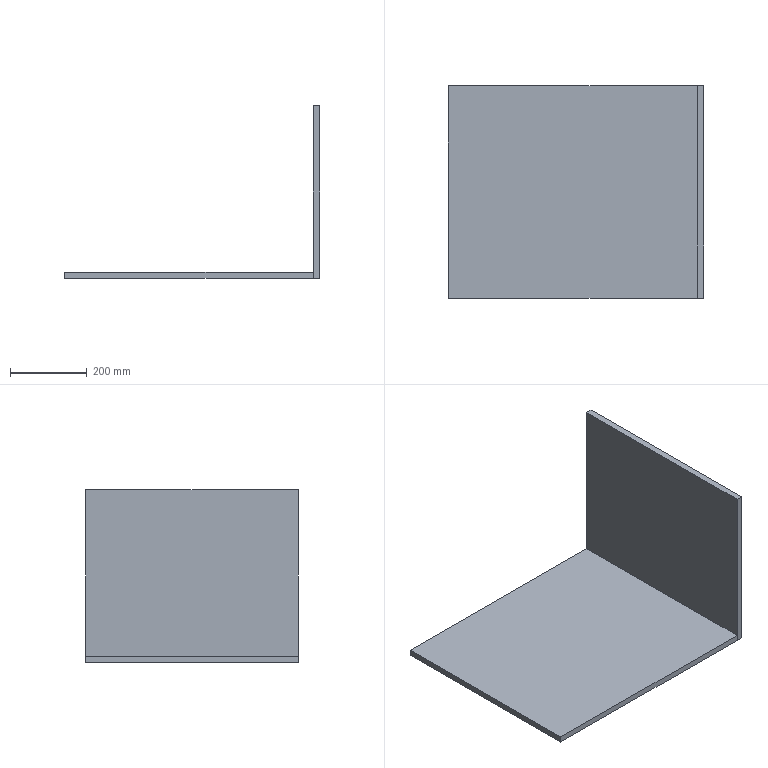Part | SolidWorks | features BaseBody 2 | 2 solids | 12 faces | box 666 x 555 x 451 mm | volume 9776880 mm3 | plane 12
STEP:
#1=CARTESIAN_POINT('',(325.,277.5,0.));
#2=VERTEX_POINT('',#1);
#3=CARTESIAN_POINT('',(-325.,277.5,0.));
#4=VERTEX_POINT('',#3);
#5=CARTESIAN_POINT('',(325.,277.5,0.));
#6=DIRECTION('',(-1.,0.,0.));
#7=VECTOR('',#6,1000.);
#8=LINE('',#5,#7);
#9=EDGE_CURVE('',#2,#4,#8,.T.);
#10=ORIENTED_EDGE('',*,*,#9,.F.);
#11=CARTESIAN_POINT('',(325.,-277.5,0.));
#12=VERTEX_POINT('',#11);
#13=CARTESIAN_POINT('',(325.,-277.5,0.));
#14=DIRECTION('',(0.,1.,0.));
#15=VECTOR('',#14,1000.);
#16=LINE('',#13,#15);
#17=EDGE_CURVE('',#12,#2,#16,.T.);
#18=ORIENTED_EDGE('',*,*,#17,.F.);
#19=CARTESIAN_POINT('',(-325.,-277.5,0.));
#20=VERTEX_POINT('',#19);
#21=CARTESIAN_POINT('',(-325.,-277.5,0.));
#22=DIRECTION('',(1.,0.,0.));
#23=VECTOR('',#22,1000.);
#24=LINE('',#21,#23);
#25=EDGE_CURVE('',#20,#12,#24,.T.);
#26=ORIENTED_EDGE('',*,*,#25,.F.);
#27=CARTESIAN_POINT('',(-325.,277.5,0.));
#28=DIRECTION('',(0.,-1.,0.));
#29=VECTOR('',#28,1000.);
#30=LINE('',#27,#29);
#31=EDGE_CURVE('',#4,#20,#30,.T.);
#32=ORIENTED_EDGE('',*,*,#31,.F.);
#33=EDGE_LOOP('',(#10,#18,#26,#32));
#34=FACE_OUTER_BOUND('',#33,.T.);
#35=CARTESIAN_POINT('',(0.,0.,0.));
#36=DIRECTION('',(0.,0.,-1.));
#37=DIRECTION('',(0.,-1.,0.));
#38=AXIS2_PLACEMENT_3D('',#35,#36,#37);
#39=PLANE('',#38);
#40=ADVANCED_FACE('',(#34),#39,.T.);
#41=CARTESIAN_POINT('',(-325.,277.5,16.));
#42=VERTEX_POINT('',#41);
#43=CARTESIAN_POINT('',(325.,277.5,16.));
#44=VERTEX_POINT('',#43);
#45=CARTESIAN_POINT('',(-325.,277.5,16.));
#46=DIRECTION('',(1.,0.,0.));
#47=VECTOR('',#46,1000.);
#48=LINE('',#45,#47);
#49=EDGE_CURVE('',#42,#44,#48,.T.);
#50=ORIENTED_EDGE('',*,*,#49,.F.);
#51=CARTESIAN_POINT('',(-325.,-277.5,16.));
#52=VERTEX_POINT('',#51);
#53=CARTESIAN_POINT('',(-325.,-277.5,16.));
#54=DIRECTION('',(0.,1.,0.));
#55=VECTOR('',#54,1000.);
#56=LINE('',#53,#55);
#57=EDGE_CURVE('',#52,#42,#56,.T.);
#58=ORIENTED_EDGE('',*,*,#57,.F.);
#59=CARTESIAN_POINT('',(325.,-277.5,16.));
#60=VERTEX_POINT('',#59);
#61=CARTESIAN_POINT('',(325.,-277.5,16.));
#62=DIRECTION('',(-1.,0.,0.));
#63=VECTOR('',#62,1000.);
#64=LINE('',#61,#63);
#65=EDGE_CURVE('',#60,#52,#64,.T.);
#66=ORIENTED_EDGE('',*,*,#65,.F.);
#67=CARTESIAN_POINT('',(325.,277.5,16.));
#68=DIRECTION('',(0.,-1.,0.));
#69=VECTOR('',#68,1000.);
#70=LINE('',#67,#69);
#71=EDGE_CURVE('',#44,#60,#70,.T.);
#72=ORIENTED_EDGE('',*,*,#71,.F.);
#73=EDGE_LOOP('',(#50,#58,#66,#72));
#74=FACE_OUTER_BOUND('',#73,.T.);
#75=CARTESIAN_POINT('',(0.,0.,16.));
#76=DIRECTION('',(0.,0.,1.));
#77=DIRECTION('',(1.,0.,0.));
#78=AXIS2_PLACEMENT_3D('',#75,#76,#77);
#79=PLANE('',#78);
#80=ADVANCED_FACE('',(#74),#79,.T.);
#81=ORIENTED_EDGE('',*,*,#9,.T.);
#82=CARTESIAN_POINT('',(-325.,277.5,16.));
#83=DIRECTION('',(0.,0.,-1.));
#84=VECTOR('',#83,1000.);
#85=LINE('',#82,#84);
#86=EDGE_CURVE('',#42,#4,#85,.T.);
#87=ORIENTED_EDGE('',*,*,#86,.F.);
#88=ORIENTED_EDGE('',*,*,#49,.T.);
#89=CARTESIAN_POINT('',(325.,277.5,0.));
#90=DIRECTION('',(0.,0.,1.));
#91=VECTOR('',#90,1000.);
#92=LINE('',#89,#91);
#93=EDGE_CURVE('',#2,#44,#92,.T.);
#94=ORIENTED_EDGE('',*,*,#93,.F.);
#95=EDGE_LOOP('',(#81,#87,#88,#94));
#96=FACE_OUTER_BOUND('',#95,.T.);
#97=CARTESIAN_POINT('',(325.,277.5,0.));
#98=DIRECTION('',(0.,1.,0.));
#99=DIRECTION('',(1.,0.,0.));
#100=AXIS2_PLACEMENT_3D('',#97,#98,#99);
#101=PLANE('',#100);
#102=ADVANCED_FACE('',(#96),#101,.T.);
#103=ORIENTED_EDGE('',*,*,#31,.T.);
#104=CARTESIAN_POINT('',(-325.,-277.5,16.));
#105=DIRECTION('',(0.,0.,-1.));
#106=VECTOR('',#105,1000.);
#107=LINE('',#104,#106);
#108=EDGE_CURVE('',#52,#20,#107,.T.);
#109=ORIENTED_EDGE('',*,*,#108,.F.);
#110=ORIENTED_EDGE('',*,*,#57,.T.);
#111=ORIENTED_EDGE('',*,*,#86,.T.);
#112=EDGE_LOOP('',(#103,#109,#110,#111));
#113=FACE_OUTER_BOUND('',#112,.T.);
#114=CARTESIAN_POINT('',(-325.,277.5,0.));
#115=DIRECTION('',(-1.,0.,0.));
#116=DIRECTION('',(0.,0.,1.));
#117=AXIS2_PLACEMENT_3D('',#114,#115,#116);
#118=PLANE('',#117);
#119=ADVANCED_FACE('',(#113),#118,.T.);
#120=ORIENTED_EDGE('',*,*,#25,.T.);
#121=CARTESIAN_POINT('',(325.,-277.5,16.));
#122=DIRECTION('',(0.,0.,-1.));
#123=VECTOR('',#122,1000.);
#124=LINE('',#121,#123);
#125=EDGE_CURVE('',#60,#12,#124,.T.);
#126=ORIENTED_EDGE('',*,*,#125,.F.);
#127=ORIENTED_EDGE('',*,*,#65,.T.);
#128=ORIENTED_EDGE('',*,*,#108,.T.);
#129=EDGE_LOOP('',(#120,#126,#127,#128));
#130=FACE_OUTER_BOUND('',#129,.T.);
#131=CARTESIAN_POINT('',(-325.,-277.5,0.));
#132=DIRECTION('',(0.,-1.,0.));
#133=DIRECTION('',(0.,0.,-1.));
#134=AXIS2_PLACEMENT_3D('',#131,#132,#133);
#135=PLANE('',#134);
#136=ADVANCED_FACE('',(#130),#135,.T.);
#137=ORIENTED_EDGE('',*,*,#17,.T.);
#138=ORIENTED_EDGE('',*,*,#93,.T.);
#139=ORIENTED_EDGE('',*,*,#71,.T.);
#140=ORIENTED_EDGE('',*,*,#125,.T.);
#141=EDGE_LOOP('',(#137,#138,#139,#140));
#142=FACE_OUTER_BOUND('',#141,.T.);
#143=CARTESIAN_POINT('',(325.,-277.5,0.));
#144=DIRECTION('',(1.,0.,0.));
#145=DIRECTION('',(0.,1.,0.));
#146=AXIS2_PLACEMENT_3D('',#143,#144,#145);
#147=PLANE('',#146);
#148=ADVANCED_FACE('',(#142),#147,.T.);
#149=CLOSED_SHELL('',(#40,#80,#102,#119,#136,#148));
#150=MANIFOLD_SOLID_BREP('',#149);
#151=CARTESIAN_POINT('',(325.,-277.5,0.));
#152=VERTEX_POINT('',#151);
#153=CARTESIAN_POINT('',(325.,277.5,0.));
#154=VERTEX_POINT('',#153);
#155=CARTESIAN_POINT('',(325.,-277.5,0.));
#156=DIRECTION('',(0.,1.,0.));
#157=VECTOR('',#156,1000.);
#158=LINE('',#155,#157);
#159=EDGE_CURVE('',#152,#154,#158,.T.);
#160=ORIENTED_EDGE('',*,*,#159,.F.);
#161=CARTESIAN_POINT('',(325.,-277.5,451.));
#162=VERTEX_POINT('',#161);
#163=CARTESIAN_POINT('',(325.,-277.5,451.));
#164=DIRECTION('',(0.,0.,-1.));
#165=VECTOR('',#164,1000.);
#166=LINE('',#163,#165);
#167=EDGE_CURVE('',#162,#152,#166,.T.);
#168=ORIENTED_EDGE('',*,*,#167,.F.);
#169=CARTESIAN_POINT('',(325.,277.5,451.));
#170=VERTEX_POINT('',#169);
#171=CARTESIAN_POINT('',(325.,277.5,451.));
#172=DIRECTION('',(0.,-1.,0.));
#173=VECTOR('',#172,1000.);
#174=LINE('',#171,#173);
#175=EDGE_CURVE('',#170,#162,#174,.T.);
#176=ORIENTED_EDGE('',*,*,#175,.F.);
#177=CARTESIAN_POINT('',(325.,277.5,0.));
#178=DIRECTION('',(0.,0.,1.));
#179=VECTOR('',#178,1000.);
#180=LINE('',#177,#179);
#181=EDGE_CURVE('',#154,#170,#180,.T.);
#182=ORIENTED_EDGE('',*,*,#181,.F.);
#183=EDGE_LOOP('',(#160,#168,#176,#182));
#184=FACE_OUTER_BOUND('',#183,.T.);
#185=CARTESIAN_POINT('',(325.,0.,225.5));
#186=DIRECTION('',(-1.,0.,0.));
#187=DIRECTION('',(0.,1.,0.));
#188=AXIS2_PLACEMENT_3D('',#185,#186,#187);
#189=PLANE('',#188);
#190=ADVANCED_FACE('',(#184),#189,.T.);
#191=CARTESIAN_POINT('',(341.,277.5,0.));
#192=VERTEX_POINT('',#191);
#193=CARTESIAN_POINT('',(341.,-277.5,0.));
#194=VERTEX_POINT('',#193);
#195=CARTESIAN_POINT('',(341.,277.5,0.));
#196=DIRECTION('',(0.,-1.,0.));
#197=VECTOR('',#196,1000.);
#198=LINE('',#195,#197);
#199=EDGE_CURVE('',#192,#194,#198,.T.);
#200=ORIENTED_EDGE('',*,*,#199,.F.);
#201=CARTESIAN_POINT('',(341.,277.5,451.));
#202=VERTEX_POINT('',#201);
#203=CARTESIAN_POINT('',(341.,277.5,451.));
#204=DIRECTION('',(0.,0.,-1.));
#205=VECTOR('',#204,1000.);
#206=LINE('',#203,#205);
#207=EDGE_CURVE('',#202,#192,#206,.T.);
#208=ORIENTED_EDGE('',*,*,#207,.F.);
#209=CARTESIAN_POINT('',(341.,-277.5,451.));
#210=VERTEX_POINT('',#209);
#211=CARTESIAN_POINT('',(341.,-277.5,451.));
#212=DIRECTION('',(0.,1.,0.));
#213=VECTOR('',#212,1000.);
#214=LINE('',#211,#213);
#215=EDGE_CURVE('',#210,#202,#214,.T.);
#216=ORIENTED_EDGE('',*,*,#215,.F.);
#217=CARTESIAN_POINT('',(341.,-277.5,0.));
#218=DIRECTION('',(0.,0.,1.));
#219=VECTOR('',#218,1000.);
#220=LINE('',#217,#219);
#221=EDGE_CURVE('',#194,#210,#220,.T.);
#222=ORIENTED_EDGE('',*,*,#221,.F.);
#223=EDGE_LOOP('',(#200,#208,#216,#222));
#224=FACE_OUTER_BOUND('',#223,.T.);
#225=CARTESIAN_POINT('',(341.,0.,225.5));
#226=DIRECTION('',(1.,0.,0.));
#227=DIRECTION('',(0.,0.,-1.));
#228=AXIS2_PLACEMENT_3D('',#225,#226,#227);
#229=PLANE('',#228);
#230=ADVANCED_FACE('',(#224),#229,.T.);
#231=ORIENTED_EDGE('',*,*,#159,.T.);
#232=CARTESIAN_POINT('',(341.,277.5,0.));
#233=DIRECTION('',(-1.,0.,0.));
#234=VECTOR('',#233,1000.);
#235=LINE('',#232,#234);
#236=EDGE_CURVE('',#192,#154,#235,.T.);
#237=ORIENTED_EDGE('',*,*,#236,.F.);
#238=ORIENTED_EDGE('',*,*,#199,.T.);
#239=CARTESIAN_POINT('',(325.,-277.5,0.));
#240=DIRECTION('',(1.,0.,0.));
#241=VECTOR('',#240,1000.);
#242=LINE('',#239,#241);
#243=EDGE_CURVE('',#152,#194,#242,.T.);
#244=ORIENTED_EDGE('',*,*,#243,.F.);
#245=EDGE_LOOP('',(#231,#237,#238,#244));
#246=FACE_OUTER_BOUND('',#245,.T.);
#247=CARTESIAN_POINT('',(325.,-277.5,0.));
#248=DIRECTION('',(0.,0.,-1.));
#249=DIRECTION('',(-1.,0.,0.));
#250=AXIS2_PLACEMENT_3D('',#247,#248,#249);
#251=PLANE('',#250);
#252=ADVANCED_FACE('',(#246),#251,.T.);
#253=ORIENTED_EDGE('',*,*,#181,.T.);
#254=CARTESIAN_POINT('',(341.,277.5,451.));
#255=DIRECTION('',(-1.,0.,0.));
#256=VECTOR('',#255,1000.);
#257=LINE('',#254,#256);
#258=EDGE_CURVE('',#202,#170,#257,.T.);
#259=ORIENTED_EDGE('',*,*,#258,.F.);
#260=ORIENTED_EDGE('',*,*,#207,.T.);
#261=ORIENTED_EDGE('',*,*,#236,.T.);
#262=EDGE_LOOP('',(#253,#259,#260,#261));
#263=FACE_OUTER_BOUND('',#262,.T.);
#264=CARTESIAN_POINT('',(325.,277.5,0.));
#265=DIRECTION('',(0.,1.,0.));
#266=DIRECTION('',(1.,0.,0.));
#267=AXIS2_PLACEMENT_3D('',#264,#265,#266);
#268=PLANE('',#267);
#269=ADVANCED_FACE('',(#263),#268,.T.);
#270=ORIENTED_EDGE('',*,*,#175,.T.);
#271=CARTESIAN_POINT('',(341.,-277.5,451.));
#272=DIRECTION('',(-1.,0.,0.));
#273=VECTOR('',#272,1000.);
#274=LINE('',#271,#273);
#275=EDGE_CURVE('',#210,#162,#274,.T.);
#276=ORIENTED_EDGE('',*,*,#275,.F.);
#277=ORIENTED_EDGE('',*,*,#215,.T.);
#278=ORIENTED_EDGE('',*,*,#258,.T.);
#279=EDGE_LOOP('',(#270,#276,#277,#278));
#280=FACE_OUTER_BOUND('',#279,.T.);
#281=CARTESIAN_POINT('',(325.,277.5,451.));
#282=DIRECTION('',(0.,0.,1.));
#283=DIRECTION('',(1.,0.,0.));
#284=AXIS2_PLACEMENT_3D('',#281,#282,#283);
#285=PLANE('',#284);
#286=ADVANCED_FACE('',(#280),#285,.T.);
#287=ORIENTED_EDGE('',*,*,#167,.T.);
#288=ORIENTED_EDGE('',*,*,#243,.T.);
#289=ORIENTED_EDGE('',*,*,#221,.T.);
#290=ORIENTED_EDGE('',*,*,#275,.T.);
#291=EDGE_LOOP('',(#287,#288,#289,#290));
#292=FACE_OUTER_BOUND('',#291,.T.);
#293=CARTESIAN_POINT('',(325.,-277.5,451.));
#294=DIRECTION('',(0.,-1.,0.));
#295=DIRECTION('',(0.,0.,-1.));
#296=AXIS2_PLACEMENT_3D('',#293,#294,#295);
#297=PLANE('',#296);
#298=ADVANCED_FACE('',(#292),#297,.T.);
#299=CLOSED_SHELL('',(#190,#230,#252,#269,#286,#298));
#300=MANIFOLD_SOLID_BREP('',#299);
#301=CARTESIAN_POINT('',(0.,0.,0.));
#302=DIRECTION('',(0.,0.,1.));
#303=DIRECTION('',(1.,0.,0.));
#304=AXIS2_PLACEMENT_3D('',#301,#302,#303);
#305=(LENGTH_UNIT()NAMED_UNIT(*)SI_UNIT(.MILLI.,.METRE.));
#306=UNCERTAINTY_MEASURE_WITH_UNIT(LENGTH_MEASURE(0.00001),#305,'','');
#307=(NAMED_UNIT(*)PLANE_ANGLE_UNIT()SI_UNIT($,.RADIAN.));
#308=(NAMED_UNIT(*)SI_UNIT($,.STERADIAN.)SOLID_ANGLE_UNIT());
#309=(GEOMETRIC_REPRESENTATION_CONTEXT(3)GLOBAL_UNCERTAINTY_ASSIGNED_CONTEXT((#306))GLOBAL_UNIT_ASSIGNED_CONTEXT((#305,#307,#308))REPRESENTATION_CONTEXT('',''));
#310=ADVANCED_BREP_SHAPE_REPRESENTATION('',(#150,#300,#304),#309);